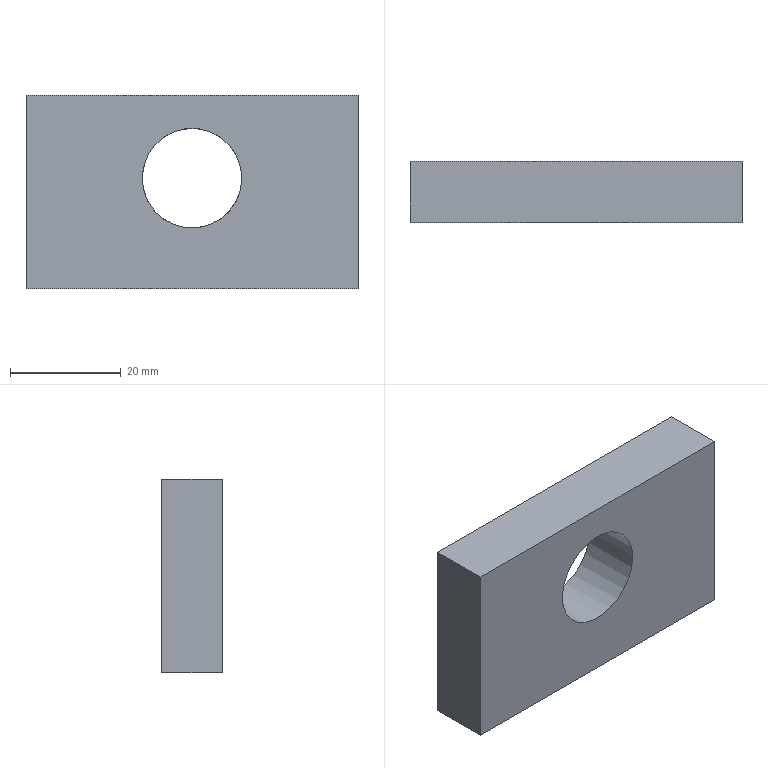Part | STEP file | solid 67 | 1 solid | 7 faces | box 60 x 11 x 35 mm | volume 20301 mm3 | plane 6 | cylinder 1 | commonest cylinder face diameters 18 x1